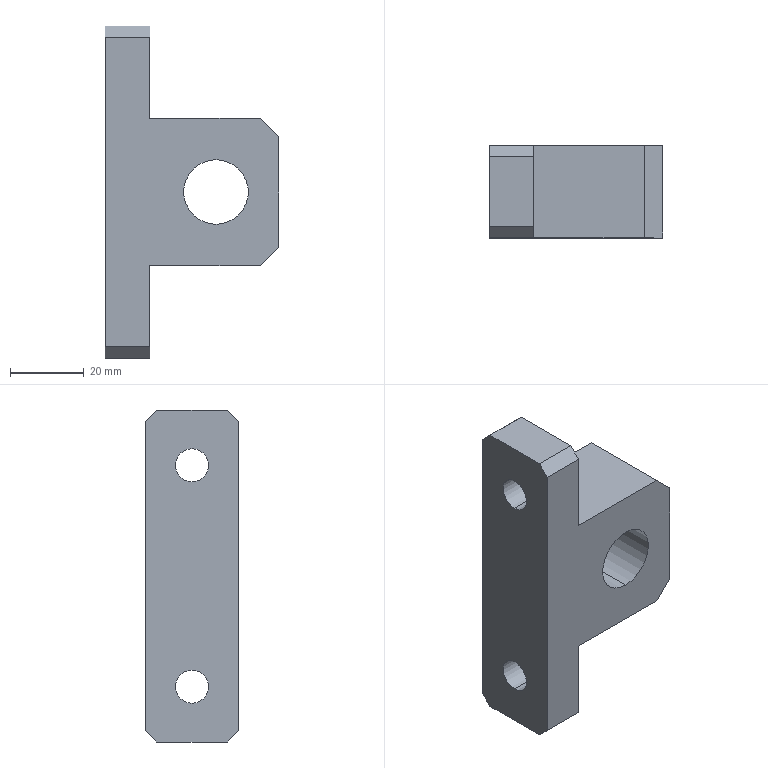Part | SolidWorks | features Chamfer 2, HoleWzd 2, Extrusion 1, ICE 1 | 1 solid | 22 faces | box 47 x 25 x 90 mm | volume 53619 mm3 | plane 16 | cylinder 6 | commonest cylinder face diameters 9 x4 17.5 x2
STEP:
#1=CARTESIAN_POINT('',(0.,0.,34.5));
#2=VERTEX_POINT('',#1);
#3=CARTESIAN_POINT('',(0.,0.,25.5));
#4=VERTEX_POINT('',#3);
#5=CARTESIAN_POINT('',(0.,0.,30.));
#6=DIRECTION('',(1.,0.,0.));
#7=DIRECTION('',(0.,0.,-1.));
#8=AXIS2_PLACEMENT_3D('',#5,#6,#7);
#9=CIRCLE('',#8,4.5);
#10=EDGE_CURVE('',#2,#4,#9,.T.);
#11=ORIENTED_EDGE('',*,*,#10,.F.);
#12=CARTESIAN_POINT('',(12.,0.,34.5));
#13=VERTEX_POINT('',#12);
#14=CARTESIAN_POINT('',(12.,0.,34.5));
#15=DIRECTION('',(1.,0.,0.));
#16=VECTOR('',#15,1000.);
#17=LINE('',#14,#16);
#18=EDGE_CURVE('',#2,#13,#17,.T.);
#19=ORIENTED_EDGE('',*,*,#18,.T.);
#20=CARTESIAN_POINT('',(12.,0.,25.5));
#21=VERTEX_POINT('',#20);
#22=CARTESIAN_POINT('',(12.,0.,30.));
#23=DIRECTION('',(1.,0.,0.));
#24=DIRECTION('',(0.,0.,-1.));
#25=AXIS2_PLACEMENT_3D('',#22,#23,#24);
#26=CIRCLE('',#25,4.5);
#27=EDGE_CURVE('',#13,#21,#26,.T.);
#28=ORIENTED_EDGE('',*,*,#27,.T.);
#29=CARTESIAN_POINT('',(12.,0.,25.5));
#30=DIRECTION('',(1.,0.,0.));
#31=VECTOR('',#30,1000.);
#32=LINE('',#29,#31);
#33=EDGE_CURVE('',#4,#21,#32,.T.);
#34=ORIENTED_EDGE('',*,*,#33,.F.);
#35=EDGE_LOOP('',(#11,#19,#28,#34));
#36=FACE_OUTER_BOUND('',#35,.T.);
#37=CARTESIAN_POINT('',(12.,0.,30.));
#38=DIRECTION('',(1.,0.,0.));
#39=DIRECTION('',(0.,0.,-1.));
#40=AXIS2_PLACEMENT_3D('',#37,#38,#39);
#41=CYLINDRICAL_SURFACE('',#40,4.5);
#42=ADVANCED_FACE('',(#36),#41,.F.);
#43=CARTESIAN_POINT('',(0.,0.,-25.5));
#44=VERTEX_POINT('',#43);
#45=CARTESIAN_POINT('',(0.,0.,-34.5));
#46=VERTEX_POINT('',#45);
#47=CARTESIAN_POINT('',(0.,0.,-30.));
#48=DIRECTION('',(1.,0.,0.));
#49=DIRECTION('',(0.,0.,-1.));
#50=AXIS2_PLACEMENT_3D('',#47,#48,#49);
#51=CIRCLE('',#50,4.5);
#52=EDGE_CURVE('',#44,#46,#51,.T.);
#53=ORIENTED_EDGE('',*,*,#52,.F.);
#54=CARTESIAN_POINT('',(12.,0.,-25.5));
#55=VERTEX_POINT('',#54);
#56=CARTESIAN_POINT('',(12.,0.,-25.5));
#57=DIRECTION('',(1.,0.,0.));
#58=VECTOR('',#57,1000.);
#59=LINE('',#56,#58);
#60=EDGE_CURVE('',#44,#55,#59,.T.);
#61=ORIENTED_EDGE('',*,*,#60,.T.);
#62=CARTESIAN_POINT('',(12.,0.,-34.5));
#63=VERTEX_POINT('',#62);
#64=CARTESIAN_POINT('',(12.,0.,-30.));
#65=DIRECTION('',(1.,0.,0.));
#66=DIRECTION('',(0.,0.,-1.));
#67=AXIS2_PLACEMENT_3D('',#64,#65,#66);
#68=CIRCLE('',#67,4.5);
#69=EDGE_CURVE('',#55,#63,#68,.T.);
#70=ORIENTED_EDGE('',*,*,#69,.T.);
#71=CARTESIAN_POINT('',(12.,0.,-34.5));
#72=DIRECTION('',(1.,0.,0.));
#73=VECTOR('',#72,1000.);
#74=LINE('',#71,#73);
#75=EDGE_CURVE('',#46,#63,#74,.T.);
#76=ORIENTED_EDGE('',*,*,#75,.F.);
#77=EDGE_LOOP('',(#53,#61,#70,#76));
#78=FACE_OUTER_BOUND('',#77,.T.);
#79=CARTESIAN_POINT('',(12.,0.,-30.));
#80=DIRECTION('',(1.,0.,0.));
#81=DIRECTION('',(0.,0.,-1.));
#82=AXIS2_PLACEMENT_3D('',#79,#80,#81);
#83=CYLINDRICAL_SURFACE('',#82,4.5);
#84=ADVANCED_FACE('',(#78),#83,.F.);
#85=CARTESIAN_POINT('',(30.,12.5,8.75));
#86=VERTEX_POINT('',#85);
#87=CARTESIAN_POINT('',(30.,12.5,-8.75));
#88=VERTEX_POINT('',#87);
#89=CARTESIAN_POINT('',(30.,12.5,0.));
#90=DIRECTION('',(0.,-1.,0.));
#91=DIRECTION('',(0.,0.,-1.));
#92=AXIS2_PLACEMENT_3D('',#89,#90,#91);
#93=CIRCLE('',#92,8.75);
#94=EDGE_CURVE('',#86,#88,#93,.T.);
#95=ORIENTED_EDGE('',*,*,#94,.F.);
#96=CARTESIAN_POINT('',(30.,-12.5,8.75));
#97=VERTEX_POINT('',#96);
#98=CARTESIAN_POINT('',(30.,-12.5,8.75));
#99=DIRECTION('',(0.,-1.,0.));
#100=VECTOR('',#99,1000.);
#101=LINE('',#98,#100);
#102=EDGE_CURVE('',#86,#97,#101,.T.);
#103=ORIENTED_EDGE('',*,*,#102,.T.);
#104=CARTESIAN_POINT('',(30.,-12.5,-8.75));
#105=VERTEX_POINT('',#104);
#106=CARTESIAN_POINT('',(30.,-12.5,0.));
#107=DIRECTION('',(0.,-1.,0.));
#108=DIRECTION('',(0.,0.,-1.));
#109=AXIS2_PLACEMENT_3D('',#106,#107,#108);
#110=CIRCLE('',#109,8.75);
#111=EDGE_CURVE('',#97,#105,#110,.T.);
#112=ORIENTED_EDGE('',*,*,#111,.T.);
#113=CARTESIAN_POINT('',(30.,-12.5,-8.75));
#114=DIRECTION('',(0.,-1.,0.));
#115=VECTOR('',#114,1000.);
#116=LINE('',#113,#115);
#117=EDGE_CURVE('',#88,#105,#116,.T.);
#118=ORIENTED_EDGE('',*,*,#117,.F.);
#119=EDGE_LOOP('',(#95,#103,#112,#118));
#120=FACE_OUTER_BOUND('',#119,.T.);
#121=CARTESIAN_POINT('',(30.,-12.5,0.));
#122=DIRECTION('',(0.,-1.,0.));
#123=DIRECTION('',(0.,0.,-1.));
#124=AXIS2_PLACEMENT_3D('',#121,#122,#123);
#125=CYLINDRICAL_SURFACE('',#124,8.75);
#126=ADVANCED_FACE('',(#120),#125,.F.);
#127=CARTESIAN_POINT('',(12.,0.,-30.));
#128=DIRECTION('',(1.,0.,0.));
#129=DIRECTION('',(0.,0.,-1.));
#130=AXIS2_PLACEMENT_3D('',#127,#128,#129);
#131=CIRCLE('',#130,4.5);
#132=EDGE_CURVE('',#63,#55,#131,.T.);
#133=ORIENTED_EDGE('',*,*,#132,.F.);
#134=ORIENTED_EDGE('',*,*,#69,.F.);
#135=EDGE_LOOP('',(#133,#134));
#136=FACE_BOUND('',#135,.T.);
#137=CARTESIAN_POINT('',(12.,-9.5,-45.));
#138=VERTEX_POINT('',#137);
#139=CARTESIAN_POINT('',(12.,9.5,-45.));
#140=VERTEX_POINT('',#139);
#141=CARTESIAN_POINT('',(12.,12.5,-45.));
#142=DIRECTION('',(0.,1.,0.));
#143=VECTOR('',#142,1000.);
#144=LINE('',#141,#143);
#145=EDGE_CURVE('',#138,#140,#144,.T.);
#146=ORIENTED_EDGE('',*,*,#145,.T.);
#147=CARTESIAN_POINT('',(12.,12.5,-42.));
#148=VERTEX_POINT('',#147);
#149=CARTESIAN_POINT('',(12.,27.25,-27.25));
#150=DIRECTION('',(0.,0.7071,0.7071));
#151=VECTOR('',#150,1000.);
#152=LINE('',#149,#151);
#153=EDGE_CURVE('',#140,#148,#152,.T.);
#154=ORIENTED_EDGE('',*,*,#153,.T.);
#155=CARTESIAN_POINT('',(12.,12.5,-20.));
#156=VERTEX_POINT('',#155);
#157=CARTESIAN_POINT('',(12.,12.5,45.));
#158=DIRECTION('',(0.,0.,1.));
#159=VECTOR('',#158,1000.);
#160=LINE('',#157,#159);
#161=EDGE_CURVE('',#148,#156,#160,.T.);
#162=ORIENTED_EDGE('',*,*,#161,.T.);
#163=CARTESIAN_POINT('',(12.,-12.5,-20.));
#164=VERTEX_POINT('',#163);
#165=CARTESIAN_POINT('',(12.,12.5,-20.));
#166=DIRECTION('',(0.,1.,0.));
#167=VECTOR('',#166,1000.);
#168=LINE('',#165,#167);
#169=EDGE_CURVE('',#164,#156,#168,.T.);
#170=ORIENTED_EDGE('',*,*,#169,.F.);
#171=CARTESIAN_POINT('',(12.,-12.5,-42.));
#172=VERTEX_POINT('',#171);
#173=CARTESIAN_POINT('',(12.,-12.5,45.));
#174=DIRECTION('',(0.,0.,-1.));
#175=VECTOR('',#174,1000.);
#176=LINE('',#173,#175);
#177=EDGE_CURVE('',#164,#172,#176,.T.);
#178=ORIENTED_EDGE('',*,*,#177,.T.);
#179=CARTESIAN_POINT('',(12.,-27.25,-27.25));
#180=DIRECTION('',(0.,0.7071,-0.7071));
#181=VECTOR('',#180,1000.);
#182=LINE('',#179,#181);
#183=EDGE_CURVE('',#172,#138,#182,.T.);
#184=ORIENTED_EDGE('',*,*,#183,.T.);
#185=EDGE_LOOP('',(#146,#154,#162,#170,#178,#184));
#186=FACE_OUTER_BOUND('',#185,.T.);
#187=CARTESIAN_POINT('',(12.,0.,0.));
#188=DIRECTION('',(1.,0.,0.));
#189=DIRECTION('',(0.,0.,-1.));
#190=AXIS2_PLACEMENT_3D('',#187,#188,#189);
#191=PLANE('',#190);
#192=ADVANCED_FACE('',(#136,#186),#191,.T.);
#193=CARTESIAN_POINT('',(0.,-9.5,-45.));
#194=VERTEX_POINT('',#193);
#195=CARTESIAN_POINT('',(0.,9.5,-45.));
#196=VERTEX_POINT('',#195);
#197=CARTESIAN_POINT('',(0.,12.5,-45.));
#198=DIRECTION('',(0.,1.,0.));
#199=VECTOR('',#198,1000.);
#200=LINE('',#197,#199);
#201=EDGE_CURVE('',#194,#196,#200,.T.);
#202=ORIENTED_EDGE('',*,*,#201,.T.);
#203=CARTESIAN_POINT('',(12.,9.5,-45.));
#204=DIRECTION('',(1.,0.,0.));
#205=VECTOR('',#204,1000.);
#206=LINE('',#203,#205);
#207=EDGE_CURVE('',#196,#140,#206,.T.);
#208=ORIENTED_EDGE('',*,*,#207,.T.);
#209=ORIENTED_EDGE('',*,*,#145,.F.);
#210=CARTESIAN_POINT('',(12.,-9.5,-45.));
#211=DIRECTION('',(-1.,0.,0.));
#212=VECTOR('',#211,1000.);
#213=LINE('',#210,#212);
#214=EDGE_CURVE('',#138,#194,#213,.T.);
#215=ORIENTED_EDGE('',*,*,#214,.T.);
#216=EDGE_LOOP('',(#202,#208,#209,#215));
#217=FACE_OUTER_BOUND('',#216,.T.);
#218=CARTESIAN_POINT('',(12.,12.5,-45.));
#219=DIRECTION('',(0.,0.,1.));
#220=DIRECTION('',(1.,0.,0.));
#221=AXIS2_PLACEMENT_3D('',#218,#219,#220);
#222=PLANE('',#221);
#223=ADVANCED_FACE('',(#217),#222,.F.);
#224=CARTESIAN_POINT('',(30.,12.5,0.));
#225=DIRECTION('',(0.,-1.,0.));
#226=DIRECTION('',(0.,0.,-1.));
#227=AXIS2_PLACEMENT_3D('',#224,#225,#226);
#228=CIRCLE('',#227,8.75);
#229=EDGE_CURVE('',#88,#86,#228,.T.);
#230=ORIENTED_EDGE('',*,*,#229,.T.);
#231=ORIENTED_EDGE('',*,*,#94,.T.);
#232=EDGE_LOOP('',(#230,#231));
#233=FACE_BOUND('',#232,.T.);
#234=ORIENTED_EDGE('',*,*,#161,.F.);
#235=CARTESIAN_POINT('',(0.,12.5,-42.));
#236=VERTEX_POINT('',#235);
#237=CARTESIAN_POINT('',(12.,12.5,-42.));
#238=DIRECTION('',(-1.,0.,0.));
#239=VECTOR('',#238,1000.);
#240=LINE('',#237,#239);
#241=EDGE_CURVE('',#148,#236,#240,.T.);
#242=ORIENTED_EDGE('',*,*,#241,.T.);
#243=CARTESIAN_POINT('',(0.,12.5,42.));
#244=VERTEX_POINT('',#243);
#245=CARTESIAN_POINT('',(0.,12.5,45.));
#246=DIRECTION('',(0.,0.,1.));
#247=VECTOR('',#246,1000.);
#248=LINE('',#245,#247);
#249=EDGE_CURVE('',#236,#244,#248,.T.);
#250=ORIENTED_EDGE('',*,*,#249,.T.);
#251=CARTESIAN_POINT('',(12.,12.5,42.));
#252=VERTEX_POINT('',#251);
#253=CARTESIAN_POINT('',(12.,12.5,42.));
#254=DIRECTION('',(1.,0.,0.));
#255=VECTOR('',#254,1000.);
#256=LINE('',#253,#255);
#257=EDGE_CURVE('',#244,#252,#256,.T.);
#258=ORIENTED_EDGE('',*,*,#257,.T.);
#259=CARTESIAN_POINT('',(12.,12.5,20.));
#260=VERTEX_POINT('',#259);
#261=CARTESIAN_POINT('',(12.,12.5,45.));
#262=DIRECTION('',(0.,0.,1.));
#263=VECTOR('',#262,1000.);
#264=LINE('',#261,#263);
#265=EDGE_CURVE('',#260,#252,#264,.T.);
#266=ORIENTED_EDGE('',*,*,#265,.F.);
#267=CARTESIAN_POINT('',(42.,12.5,20.));
#268=VERTEX_POINT('',#267);
#269=CARTESIAN_POINT('',(47.,12.5,20.));
#270=DIRECTION('',(-1.,0.,0.));
#271=VECTOR('',#270,1000.);
#272=LINE('',#269,#271);
#273=EDGE_CURVE('',#268,#260,#272,.T.);
#274=ORIENTED_EDGE('',*,*,#273,.F.);
#275=CARTESIAN_POINT('',(47.,12.5,15.));
#276=VERTEX_POINT('',#275);
#277=CARTESIAN_POINT('',(47.,12.5,15.));
#278=DIRECTION('',(0.7071,0.,-0.7071));
#279=VECTOR('',#278,1000.);
#280=LINE('',#277,#279);
#281=EDGE_CURVE('',#268,#276,#280,.T.);
#282=ORIENTED_EDGE('',*,*,#281,.T.);
#283=CARTESIAN_POINT('',(47.,12.5,-15.));
#284=VERTEX_POINT('',#283);
#285=CARTESIAN_POINT('',(47.,12.5,20.));
#286=DIRECTION('',(0.,0.,1.));
#287=VECTOR('',#286,1000.);
#288=LINE('',#285,#287);
#289=EDGE_CURVE('',#284,#276,#288,.T.);
#290=ORIENTED_EDGE('',*,*,#289,.F.);
#291=CARTESIAN_POINT('',(42.,12.5,-20.));
#292=VERTEX_POINT('',#291);
#293=CARTESIAN_POINT('',(47.,12.5,-15.));
#294=DIRECTION('',(-0.7071,0.,-0.7071));
#295=VECTOR('',#294,1000.);
#296=LINE('',#293,#295);
#297=EDGE_CURVE('',#284,#292,#296,.T.);
#298=ORIENTED_EDGE('',*,*,#297,.T.);
#299=CARTESIAN_POINT('',(47.,12.5,-20.));
#300=DIRECTION('',(-1.,0.,0.));
#301=VECTOR('',#300,1000.);
#302=LINE('',#299,#301);
#303=EDGE_CURVE('',#292,#156,#302,.T.);
#304=ORIENTED_EDGE('',*,*,#303,.T.);
#305=EDGE_LOOP('',(#234,#242,#250,#258,#266,#274,#282,#290,#298,#304));
#306=FACE_OUTER_BOUND('',#305,.T.);
#307=CARTESIAN_POINT('',(12.,12.5,45.));
#308=DIRECTION('',(0.,-1.,0.));
#309=DIRECTION('',(0.,0.,-1.));
#310=AXIS2_PLACEMENT_3D('',#307,#308,#309);
#311=PLANE('',#310);
#312=ADVANCED_FACE('',(#233,#306),#311,.F.);
#313=CARTESIAN_POINT('',(12.,9.5,45.));
#314=VERTEX_POINT('',#313);
#315=CARTESIAN_POINT('',(12.,-9.5,45.));
#316=VERTEX_POINT('',#315);
#317=CARTESIAN_POINT('',(12.,12.5,45.));
#318=DIRECTION('',(0.,-1.,0.));
#319=VECTOR('',#318,1000.);
#320=LINE('',#317,#319);
#321=EDGE_CURVE('',#314,#316,#320,.T.);
#322=ORIENTED_EDGE('',*,*,#321,.F.);
#323=CARTESIAN_POINT('',(0.,9.5,45.));
#324=VERTEX_POINT('',#323);
#325=CARTESIAN_POINT('',(12.,9.5,45.));
#326=DIRECTION('',(-1.,0.,0.));
#327=VECTOR('',#326,1000.);
#328=LINE('',#325,#327);
#329=EDGE_CURVE('',#314,#324,#328,.T.);
#330=ORIENTED_EDGE('',*,*,#329,.T.);
#331=CARTESIAN_POINT('',(0.,-9.5,45.));
#332=VERTEX_POINT('',#331);
#333=CARTESIAN_POINT('',(0.,12.5,45.));
#334=DIRECTION('',(0.,-1.,0.));
#335=VECTOR('',#334,1000.);
#336=LINE('',#333,#335);
#337=EDGE_CURVE('',#324,#332,#336,.T.);
#338=ORIENTED_EDGE('',*,*,#337,.T.);
#339=CARTESIAN_POINT('',(12.,-9.5,45.));
#340=DIRECTION('',(1.,0.,0.));
#341=VECTOR('',#340,1000.);
#342=LINE('',#339,#341);
#343=EDGE_CURVE('',#332,#316,#342,.T.);
#344=ORIENTED_EDGE('',*,*,#343,.T.);
#345=EDGE_LOOP('',(#322,#330,#338,#344));
#346=FACE_OUTER_BOUND('',#345,.T.);
#347=CARTESIAN_POINT('',(12.,12.5,45.));
#348=DIRECTION('',(0.,0.,-1.));
#349=DIRECTION('',(-1.,0.,0.));
#350=AXIS2_PLACEMENT_3D('',#347,#348,#349);
#351=PLANE('',#350);
#352=ADVANCED_FACE('',(#346),#351,.F.);
#353=CARTESIAN_POINT('',(30.,-12.5,0.));
#354=DIRECTION('',(0.,-1.,0.));
#355=DIRECTION('',(0.,0.,-1.));
#356=AXIS2_PLACEMENT_3D('',#353,#354,#355);
#357=CIRCLE('',#356,8.75);
#358=EDGE_CURVE('',#105,#97,#357,.T.);
#359=ORIENTED_EDGE('',*,*,#358,.F.);
#360=ORIENTED_EDGE('',*,*,#111,.F.);
#361=EDGE_LOOP('',(#359,#360));
#362=FACE_BOUND('',#361,.T.);
#363=CARTESIAN_POINT('',(0.,-12.5,42.));
#364=VERTEX_POINT('',#363);
#365=CARTESIAN_POINT('',(0.,-12.5,-42.));
#366=VERTEX_POINT('',#365);
#367=CARTESIAN_POINT('',(0.,-12.5,45.));
#368=DIRECTION('',(0.,0.,-1.));
#369=VECTOR('',#368,1000.);
#370=LINE('',#367,#369);
#371=EDGE_CURVE('',#364,#366,#370,.T.);
#372=ORIENTED_EDGE('',*,*,#371,.T.);
#373=CARTESIAN_POINT('',(12.,-12.5,-42.));
#374=DIRECTION('',(1.,0.,0.));
#375=VECTOR('',#374,1000.);
#376=LINE('',#373,#375);
#377=EDGE_CURVE('',#366,#172,#376,.T.);
#378=ORIENTED_EDGE('',*,*,#377,.T.);
#379=ORIENTED_EDGE('',*,*,#177,.F.);
#380=CARTESIAN_POINT('',(42.,-12.5,-20.));
#381=VERTEX_POINT('',#380);
#382=CARTESIAN_POINT('',(47.,-12.5,-20.));
#383=DIRECTION('',(-1.,0.,0.));
#384=VECTOR('',#383,1000.);
#385=LINE('',#382,#384);
#386=EDGE_CURVE('',#381,#164,#385,.T.);
#387=ORIENTED_EDGE('',*,*,#386,.F.);
#388=CARTESIAN_POINT('',(47.,-12.5,-15.));
#389=VERTEX_POINT('',#388);
#390=CARTESIAN_POINT('',(47.,-12.5,-15.));
#391=DIRECTION('',(0.7071,0.,0.7071));
#392=VECTOR('',#391,1000.);
#393=LINE('',#390,#392);
#394=EDGE_CURVE('',#381,#389,#393,.T.);
#395=ORIENTED_EDGE('',*,*,#394,.T.);
#396=CARTESIAN_POINT('',(47.,-12.5,15.));
#397=VERTEX_POINT('',#396);
#398=CARTESIAN_POINT('',(47.,-12.5,20.));
#399=DIRECTION('',(0.,0.,-1.));
#400=VECTOR('',#399,1000.);
#401=LINE('',#398,#400);
#402=EDGE_CURVE('',#397,#389,#401,.T.);
#403=ORIENTED_EDGE('',*,*,#402,.F.);
#404=CARTESIAN_POINT('',(42.,-12.5,20.));
#405=VERTEX_POINT('',#404);
#406=CARTESIAN_POINT('',(47.,-12.5,15.));
#407=DIRECTION('',(-0.7071,0.,0.7071));
#408=VECTOR('',#407,1000.);
#409=LINE('',#406,#408);
#410=EDGE_CURVE('',#397,#405,#409,.T.);
#411=ORIENTED_EDGE('',*,*,#410,.T.);
#412=CARTESIAN_POINT('',(12.,-12.5,20.));
#413=VERTEX_POINT('',#412);
#414=CARTESIAN_POINT('',(47.,-12.5,20.));
#415=DIRECTION('',(-1.,0.,0.));
#416=VECTOR('',#415,1000.);
#417=LINE('',#414,#416);
#418=EDGE_CURVE('',#405,#413,#417,.T.);
#419=ORIENTED_EDGE('',*,*,#418,.T.);
#420=CARTESIAN_POINT('',(12.,-12.5,42.));
#421=VERTEX_POINT('',#420);
#422=CARTESIAN_POINT('',(12.,-12.5,45.));
#423=DIRECTION('',(0.,0.,-1.));
#424=VECTOR('',#423,1000.);
#425=LINE('',#422,#424);
#426=EDGE_CURVE('',#421,#413,#425,.T.);
#427=ORIENTED_EDGE('',*,*,#426,.F.);
#428=CARTESIAN_POINT('',(12.,-12.5,42.));
#429=DIRECTION('',(-1.,0.,0.));
#430=VECTOR('',#429,1000.);
#431=LINE('',#428,#430);
#432=EDGE_CURVE('',#421,#364,#431,.T.);
#433=ORIENTED_EDGE('',*,*,#432,.T.);
#434=EDGE_LOOP('',(#372,#378,#379,#387,#395,#403,#411,#419,#427,#433));
#435=FACE_OUTER_BOUND('',#434,.T.);
#436=CARTESIAN_POINT('',(12.,-12.5,45.));
#437=DIRECTION('',(0.,1.,0.));
#438=DIRECTION('',(0.,0.,1.));
#439=AXIS2_PLACEMENT_3D('',#436,#437,#438);
#440=PLANE('',#439);
#441=ADVANCED_FACE('',(#362,#435),#440,.F.);
#442=CARTESIAN_POINT('',(12.,0.,30.));
#443=DIRECTION('',(1.,0.,0.));
#444=DIRECTION('',(0.,0.,-1.));
#445=AXIS2_PLACEMENT_3D('',#442,#443,#444);
#446=CIRCLE('',#445,4.5);
#447=EDGE_CURVE('',#21,#13,#446,.T.);
#448=ORIENTED_EDGE('',*,*,#447,.F.);
#449=ORIENTED_EDGE('',*,*,#27,.F.);
#450=EDGE_LOOP('',(#448,#449));
#451=FACE_BOUND('',#450,.T.);
#452=ORIENTED_EDGE('',*,*,#265,.T.);
#453=CARTESIAN_POINT('',(12.,27.25,27.25));
#454=DIRECTION('',(0.,-0.7071,0.7071));
#455=VECTOR('',#454,1000.);
#456=LINE('',#453,#455);
#457=EDGE_CURVE('',#252,#314,#456,.T.);
#458=ORIENTED_EDGE('',*,*,#457,.T.);
#459=ORIENTED_EDGE('',*,*,#321,.T.);
#460=CARTESIAN_POINT('',(12.,-27.25,27.25));
#461=DIRECTION('',(0.,-0.7071,-0.7071));
#462=VECTOR('',#461,1000.);
#463=LINE('',#460,#462);
#464=EDGE_CURVE('',#316,#421,#463,.T.);
#465=ORIENTED_EDGE('',*,*,#464,.T.);
#466=ORIENTED_EDGE('',*,*,#426,.T.);
#467=CARTESIAN_POINT('',(12.,12.5,20.));
#468=DIRECTION('',(0.,-1.,0.));
#469=VECTOR('',#468,1000.);
#470=LINE('',#467,#469);
#471=EDGE_CURVE('',#260,#413,#470,.T.);
#472=ORIENTED_EDGE('',*,*,#471,.F.);
#473=EDGE_LOOP('',(#452,#458,#459,#465,#466,#472));
#474=FACE_OUTER_BOUND('',#473,.T.);
#475=CARTESIAN_POINT('',(12.,0.,0.));
#476=DIRECTION('',(1.,0.,0.));
#477=DIRECTION('',(0.,0.,-1.));
#478=AXIS2_PLACEMENT_3D('',#475,#476,#477);
#479=PLANE('',#478);
#480=ADVANCED_FACE('',(#451,#474),#479,.T.);
#481=CARTESIAN_POINT('',(0.,0.,30.));
#482=DIRECTION('',(1.,0.,0.));
#483=DIRECTION('',(0.,0.,-1.));
#484=AXIS2_PLACEMENT_3D('',#481,#482,#483);
#485=CIRCLE('',#484,4.5);
#486=EDGE_CURVE('',#4,#2,#485,.T.);
#487=ORIENTED_EDGE('',*,*,#486,.T.);
#488=ORIENTED_EDGE('',*,*,#10,.T.);
#489=EDGE_LOOP('',(#487,#488));
#490=FACE_BOUND('',#489,.T.);
#491=CARTESIAN_POINT('',(0.,0.,-30.));
#492=DIRECTION('',(1.,0.,0.));
#493=DIRECTION('',(0.,0.,-1.));
#494=AXIS2_PLACEMENT_3D('',#491,#492,#493);
#495=CIRCLE('',#494,4.5);
#496=EDGE_CURVE('',#46,#44,#495,.T.);
#497=ORIENTED_EDGE('',*,*,#496,.T.);
#498=ORIENTED_EDGE('',*,*,#52,.T.);
#499=EDGE_LOOP('',(#497,#498));
#500=FACE_BOUND('',#499,.T.);
#501=ORIENTED_EDGE('',*,*,#249,.F.);
#502=CARTESIAN_POINT('',(0.,12.5,-42.));
#503=DIRECTION('',(0.,-0.7071,-0.7071));
#504=VECTOR('',#503,1000.);
#505=LINE('',#502,#504);
#506=EDGE_CURVE('',#236,#196,#505,.T.);
#507=ORIENTED_EDGE('',*,*,#506,.T.);
#508=ORIENTED_EDGE('',*,*,#201,.F.);
#509=CARTESIAN_POINT('',(0.,-9.5,-45.));
#510=DIRECTION('',(0.,-0.7071,0.7071));
#511=VECTOR('',#510,1000.);
#512=LINE('',#509,#511);
#513=EDGE_CURVE('',#194,#366,#512,.T.);
#514=ORIENTED_EDGE('',*,*,#513,.T.);
#515=ORIENTED_EDGE('',*,*,#371,.F.);
#516=CARTESIAN_POINT('',(0.,-12.5,42.));
#517=DIRECTION('',(0.,0.7071,0.7071));
#518=VECTOR('',#517,1000.);
#519=LINE('',#516,#518);
#520=EDGE_CURVE('',#364,#332,#519,.T.);
#521=ORIENTED_EDGE('',*,*,#520,.T.);
#522=ORIENTED_EDGE('',*,*,#337,.F.);
#523=CARTESIAN_POINT('',(0.,9.5,45.));
#524=DIRECTION('',(0.,0.7071,-0.7071));
#525=VECTOR('',#524,1000.);
#526=LINE('',#523,#525);
#527=EDGE_CURVE('',#324,#244,#526,.T.);
#528=ORIENTED_EDGE('',*,*,#527,.T.);
#529=EDGE_LOOP('',(#501,#507,#508,#514,#515,#521,#522,#528));
#530=FACE_OUTER_BOUND('',#529,.T.);
#531=CARTESIAN_POINT('',(0.,0.,0.));
#532=DIRECTION('',(1.,0.,0.));
#533=DIRECTION('',(0.,0.,-1.));
#534=AXIS2_PLACEMENT_3D('',#531,#532,#533);
#535=PLANE('',#534);
#536=ADVANCED_FACE('',(#490,#500,#530),#535,.F.);
#537=ORIENTED_EDGE('',*,*,#303,.F.);
#538=CARTESIAN_POINT('',(42.,-12.5,-20.));
#539=DIRECTION('',(0.,-1.,0.));
#540=VECTOR('',#539,1000.);
#541=LINE('',#538,#540);
#542=EDGE_CURVE('',#292,#381,#541,.T.);
#543=ORIENTED_EDGE('',*,*,#542,.T.);
#544=ORIENTED_EDGE('',*,*,#386,.T.);
#545=ORIENTED_EDGE('',*,*,#169,.T.);
#546=EDGE_LOOP('',(#537,#543,#544,#545));
#547=FACE_OUTER_BOUND('',#546,.T.);
#548=CARTESIAN_POINT('',(47.,12.5,-20.));
#549=DIRECTION('',(0.,0.,1.));
#550=DIRECTION('',(1.,0.,0.));
#551=AXIS2_PLACEMENT_3D('',#548,#549,#550);
#552=PLANE('',#551);
#553=ADVANCED_FACE('',(#547),#552,.F.);
#554=ORIENTED_EDGE('',*,*,#418,.F.);
#555=CARTESIAN_POINT('',(42.,12.5,20.));
#556=DIRECTION('',(0.,1.,0.));
#557=VECTOR('',#556,1000.);
#558=LINE('',#555,#557);
#559=EDGE_CURVE('',#405,#268,#558,.T.);
#560=ORIENTED_EDGE('',*,*,#559,.T.);
#561=ORIENTED_EDGE('',*,*,#273,.T.);
#562=ORIENTED_EDGE('',*,*,#471,.T.);
#563=EDGE_LOOP('',(#554,#560,#561,#562));
#564=FACE_OUTER_BOUND('',#563,.T.);
#565=CARTESIAN_POINT('',(47.,12.5,20.));
#566=DIRECTION('',(0.,0.,-1.));
#567=DIRECTION('',(0.,1.,0.));
#568=AXIS2_PLACEMENT_3D('',#565,#566,#567);
#569=PLANE('',#568);
#570=ADVANCED_FACE('',(#564),#569,.F.);
#571=ORIENTED_EDGE('',*,*,#402,.T.);
#572=CARTESIAN_POINT('',(47.,12.5,-15.));
#573=DIRECTION('',(0.,1.,0.));
#574=VECTOR('',#573,1000.);
#575=LINE('',#572,#574);
#576=EDGE_CURVE('',#389,#284,#575,.T.);
#577=ORIENTED_EDGE('',*,*,#576,.T.);
#578=ORIENTED_EDGE('',*,*,#289,.T.);
#579=CARTESIAN_POINT('',(47.,-12.5,15.));
#580=DIRECTION('',(0.,-1.,0.));
#581=VECTOR('',#580,1000.);
#582=LINE('',#579,#581);
#583=EDGE_CURVE('',#276,#397,#582,.T.);
#584=ORIENTED_EDGE('',*,*,#583,.T.);
#585=EDGE_LOOP('',(#571,#577,#578,#584));
#586=FACE_OUTER_BOUND('',#585,.T.);
#587=CARTESIAN_POINT('',(47.,0.,0.));
#588=DIRECTION('',(1.,0.,0.));
#589=DIRECTION('',(0.,0.,-1.));
#590=AXIS2_PLACEMENT_3D('',#587,#588,#589);
#591=PLANE('',#590);
#592=ADVANCED_FACE('',(#586),#591,.T.);
#593=ORIENTED_EDGE('',*,*,#102,.F.);
#594=ORIENTED_EDGE('',*,*,#229,.F.);
#595=ORIENTED_EDGE('',*,*,#117,.T.);
#596=ORIENTED_EDGE('',*,*,#358,.T.);
#597=EDGE_LOOP('',(#593,#594,#595,#596));
#598=FACE_OUTER_BOUND('',#597,.T.);
#599=CARTESIAN_POINT('',(30.,-12.5,0.));
#600=DIRECTION('',(0.,-1.,0.));
#601=DIRECTION('',(0.,0.,-1.));
#602=AXIS2_PLACEMENT_3D('',#599,#600,#601);
#603=CYLINDRICAL_SURFACE('',#602,8.75);
#604=ADVANCED_FACE('',(#598),#603,.F.);
#605=ORIENTED_EDGE('',*,*,#60,.F.);
#606=ORIENTED_EDGE('',*,*,#496,.F.);
#607=ORIENTED_EDGE('',*,*,#75,.T.);
#608=ORIENTED_EDGE('',*,*,#132,.T.);
#609=EDGE_LOOP('',(#605,#606,#607,#608));
#610=FACE_OUTER_BOUND('',#609,.T.);
#611=CARTESIAN_POINT('',(12.,0.,-30.));
#612=DIRECTION('',(1.,0.,0.));
#613=DIRECTION('',(0.,0.,-1.));
#614=AXIS2_PLACEMENT_3D('',#611,#612,#613);
#615=CYLINDRICAL_SURFACE('',#614,4.5);
#616=ADVANCED_FACE('',(#610),#615,.F.);
#617=ORIENTED_EDGE('',*,*,#18,.F.);
#618=ORIENTED_EDGE('',*,*,#486,.F.);
#619=ORIENTED_EDGE('',*,*,#33,.T.);
#620=ORIENTED_EDGE('',*,*,#447,.T.);
#621=EDGE_LOOP('',(#617,#618,#619,#620));
#622=FACE_OUTER_BOUND('',#621,.T.);
#623=CARTESIAN_POINT('',(12.,0.,30.));
#624=DIRECTION('',(1.,0.,0.));
#625=DIRECTION('',(0.,0.,-1.));
#626=AXIS2_PLACEMENT_3D('',#623,#624,#625);
#627=CYLINDRICAL_SURFACE('',#626,4.5);
#628=ADVANCED_FACE('',(#622),#627,.F.);
#629=ORIENTED_EDGE('',*,*,#394,.F.);
#630=ORIENTED_EDGE('',*,*,#542,.F.);
#631=ORIENTED_EDGE('',*,*,#297,.F.);
#632=ORIENTED_EDGE('',*,*,#576,.F.);
#633=EDGE_LOOP('',(#629,#630,#631,#632));
#634=FACE_OUTER_BOUND('',#633,.T.);
#635=CARTESIAN_POINT('',(47.,0.,-15.));
#636=DIRECTION('',(0.7071,0.,-0.7071));
#637=DIRECTION('',(0.,-1.,0.));
#638=AXIS2_PLACEMENT_3D('',#635,#636,#637);
#639=PLANE('',#638);
#640=ADVANCED_FACE('',(#634),#639,.T.);
#641=ORIENTED_EDGE('',*,*,#281,.F.);
#642=ORIENTED_EDGE('',*,*,#559,.F.);
#643=ORIENTED_EDGE('',*,*,#410,.F.);
#644=ORIENTED_EDGE('',*,*,#583,.F.);
#645=EDGE_LOOP('',(#641,#642,#643,#644));
#646=FACE_OUTER_BOUND('',#645,.T.);
#647=CARTESIAN_POINT('',(47.,0.,15.));
#648=DIRECTION('',(0.7071,0.,0.7071));
#649=DIRECTION('',(0.,1.,0.));
#650=AXIS2_PLACEMENT_3D('',#647,#648,#649);
#651=PLANE('',#650);
#652=ADVANCED_FACE('',(#646),#651,.T.);
#653=ORIENTED_EDGE('',*,*,#153,.F.);
#654=ORIENTED_EDGE('',*,*,#207,.F.);
#655=ORIENTED_EDGE('',*,*,#506,.F.);
#656=ORIENTED_EDGE('',*,*,#241,.F.);
#657=EDGE_LOOP('',(#653,#654,#655,#656));
#658=FACE_OUTER_BOUND('',#657,.T.);
#659=CARTESIAN_POINT('',(12.,12.5,-42.));
#660=DIRECTION('',(0.,-0.7071,0.7071));
#661=DIRECTION('',(-1.,0.,0.));
#662=AXIS2_PLACEMENT_3D('',#659,#660,#661);
#663=PLANE('',#662);
#664=ADVANCED_FACE('',(#658),#663,.F.);
#665=ORIENTED_EDGE('',*,*,#183,.F.);
#666=ORIENTED_EDGE('',*,*,#377,.F.);
#667=ORIENTED_EDGE('',*,*,#513,.F.);
#668=ORIENTED_EDGE('',*,*,#214,.F.);
#669=EDGE_LOOP('',(#665,#666,#667,#668));
#670=FACE_OUTER_BOUND('',#669,.T.);
#671=CARTESIAN_POINT('',(12.,-9.5,-45.));
#672=DIRECTION('',(0.,0.7071,0.7071));
#673=DIRECTION('',(-1.,0.,0.));
#674=AXIS2_PLACEMENT_3D('',#671,#672,#673);
#675=PLANE('',#674);
#676=ADVANCED_FACE('',(#670),#675,.F.);
#677=ORIENTED_EDGE('',*,*,#457,.F.);
#678=ORIENTED_EDGE('',*,*,#257,.F.);
#679=ORIENTED_EDGE('',*,*,#527,.F.);
#680=ORIENTED_EDGE('',*,*,#329,.F.);
#681=EDGE_LOOP('',(#677,#678,#679,#680));
#682=FACE_OUTER_BOUND('',#681,.T.);
#683=CARTESIAN_POINT('',(12.,9.5,45.));
#684=DIRECTION('',(0.,-0.7071,-0.7071));
#685=DIRECTION('',(-1.,0.,0.));
#686=AXIS2_PLACEMENT_3D('',#683,#684,#685);
#687=PLANE('',#686);
#688=ADVANCED_FACE('',(#682),#687,.F.);
#689=ORIENTED_EDGE('',*,*,#464,.F.);
#690=ORIENTED_EDGE('',*,*,#343,.F.);
#691=ORIENTED_EDGE('',*,*,#520,.F.);
#692=ORIENTED_EDGE('',*,*,#432,.F.);
#693=EDGE_LOOP('',(#689,#690,#691,#692));
#694=FACE_OUTER_BOUND('',#693,.T.);
#695=CARTESIAN_POINT('',(12.,-12.5,42.));
#696=DIRECTION('',(0.,0.7071,-0.7071));
#697=DIRECTION('',(-1.,0.,0.));
#698=AXIS2_PLACEMENT_3D('',#695,#696,#697);
#699=PLANE('',#698);
#700=ADVANCED_FACE('',(#694),#699,.F.);
#701=CLOSED_SHELL('',(#42,#84,#126,#192,#223,#312,#352,#441,#480,#536,#553,#570,#592,#604,#616,#628,#640,#652,#664,#676,#688,#700));
#702=MANIFOLD_SOLID_BREP('',#701);
#703=CARTESIAN_POINT('',(0.,0.,0.));
#704=DIRECTION('',(0.,0.,1.));
#705=DIRECTION('',(1.,0.,0.));
#706=AXIS2_PLACEMENT_3D('',#703,#704,#705);
#707=(LENGTH_UNIT()NAMED_UNIT(*)SI_UNIT(.MILLI.,.METRE.));
#708=UNCERTAINTY_MEASURE_WITH_UNIT(LENGTH_MEASURE(0.00001),#707,'','');
#709=(NAMED_UNIT(*)PLANE_ANGLE_UNIT()SI_UNIT($,.RADIAN.));
#710=(NAMED_UNIT(*)SI_UNIT($,.STERADIAN.)SOLID_ANGLE_UNIT());
#711=(GEOMETRIC_REPRESENTATION_CONTEXT(3)GLOBAL_UNCERTAINTY_ASSIGNED_CONTEXT((#708))GLOBAL_UNIT_ASSIGNED_CONTEXT((#707,#709,#710))REPRESENTATION_CONTEXT('',''));
#712=ADVANCED_BREP_SHAPE_REPRESENTATION('',(#702,#706),#711);